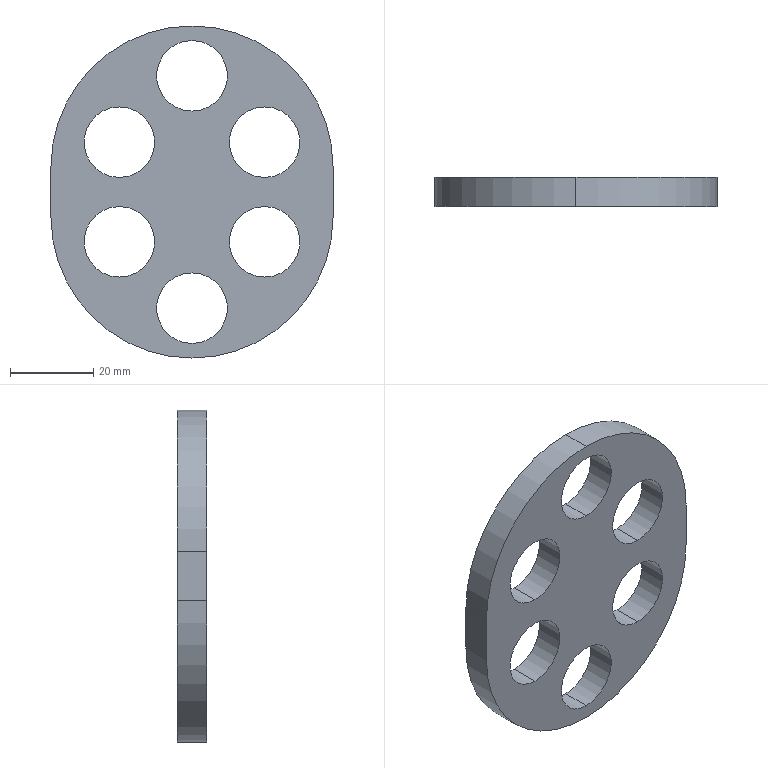Part | SolidWorks | features MirrorStock 1 | 1 solid | 19 faces | box 68 x 7 x 80 mm | volume 21601 mm3 | cylinder 15 | plane 4 | commonest cylinder face diameters 17 x12 68 x3
STEP:
#1=CARTESIAN_POINT('',(0.,7.,-36.5));
#2=VERTEX_POINT('',#1);
#3=CARTESIAN_POINT('',(0.,7.,-19.5));
#4=VERTEX_POINT('',#3);
#5=CARTESIAN_POINT('',(0.,7.,-28.));
#6=DIRECTION('',(0.,-1.,0.));
#7=DIRECTION('',(0.,0.,1.));
#8=AXIS2_PLACEMENT_3D('',#5,#6,#7);
#9=CIRCLE('',#8,8.5);
#10=EDGE_CURVE('',#2,#4,#9,.T.);
#11=ORIENTED_EDGE('',*,*,#10,.F.);
#12=CARTESIAN_POINT('',(0.,0.,-36.5));
#13=VERTEX_POINT('',#12);
#14=CARTESIAN_POINT('',(0.,7.,-36.5));
#15=DIRECTION('',(0.,-1.,0.));
#16=VECTOR('',#15,1000.);
#17=LINE('',#14,#16);
#18=EDGE_CURVE('',#2,#13,#17,.T.);
#19=ORIENTED_EDGE('',*,*,#18,.T.);
#20=CARTESIAN_POINT('',(0.,0.,-19.5));
#21=VERTEX_POINT('',#20);
#22=CARTESIAN_POINT('',(0.,0.,-28.));
#23=DIRECTION('',(0.,-1.,0.));
#24=DIRECTION('',(0.,0.,1.));
#25=AXIS2_PLACEMENT_3D('',#22,#23,#24);
#26=CIRCLE('',#25,8.5);
#27=EDGE_CURVE('',#13,#21,#26,.T.);
#28=ORIENTED_EDGE('',*,*,#27,.T.);
#29=CARTESIAN_POINT('',(0.,7.,-19.5));
#30=DIRECTION('',(0.,-1.,0.));
#31=VECTOR('',#30,1000.);
#32=LINE('',#29,#31);
#33=EDGE_CURVE('',#4,#21,#32,.T.);
#34=ORIENTED_EDGE('',*,*,#33,.F.);
#35=EDGE_LOOP('',(#11,#19,#28,#34));
#36=FACE_OUTER_BOUND('',#35,.T.);
#37=CARTESIAN_POINT('',(0.,7.,-28.));
#38=DIRECTION('',(0.,-1.,0.));
#39=DIRECTION('',(0.,0.,1.));
#40=AXIS2_PLACEMENT_3D('',#37,#38,#39);
#41=CYLINDRICAL_SURFACE('',#40,8.5);
#42=ADVANCED_FACE('',(#36),#41,.F.);
#43=CARTESIAN_POINT('',(-17.5,7.,-20.5));
#44=VERTEX_POINT('',#43);
#45=CARTESIAN_POINT('',(-17.5,7.,-3.5));
#46=VERTEX_POINT('',#45);
#47=CARTESIAN_POINT('',(-17.5,7.,-12.));
#48=DIRECTION('',(0.,-1.,0.));
#49=DIRECTION('',(0.,0.,1.));
#50=AXIS2_PLACEMENT_3D('',#47,#48,#49);
#51=CIRCLE('',#50,8.5);
#52=EDGE_CURVE('',#44,#46,#51,.T.);
#53=ORIENTED_EDGE('',*,*,#52,.F.);
#54=CARTESIAN_POINT('',(-17.5,0.,-20.5));
#55=VERTEX_POINT('',#54);
#56=CARTESIAN_POINT('',(-17.5,7.,-20.5));
#57=DIRECTION('',(0.,-1.,0.));
#58=VECTOR('',#57,1000.);
#59=LINE('',#56,#58);
#60=EDGE_CURVE('',#44,#55,#59,.T.);
#61=ORIENTED_EDGE('',*,*,#60,.T.);
#62=CARTESIAN_POINT('',(-17.5,0.,-3.5));
#63=VERTEX_POINT('',#62);
#64=CARTESIAN_POINT('',(-17.5,0.,-12.));
#65=DIRECTION('',(0.,-1.,0.));
#66=DIRECTION('',(0.,0.,1.));
#67=AXIS2_PLACEMENT_3D('',#64,#65,#66);
#68=CIRCLE('',#67,8.5);
#69=EDGE_CURVE('',#55,#63,#68,.T.);
#70=ORIENTED_EDGE('',*,*,#69,.T.);
#71=CARTESIAN_POINT('',(-17.5,7.,-3.5));
#72=DIRECTION('',(0.,-1.,0.));
#73=VECTOR('',#72,1000.);
#74=LINE('',#71,#73);
#75=EDGE_CURVE('',#46,#63,#74,.T.);
#76=ORIENTED_EDGE('',*,*,#75,.F.);
#77=EDGE_LOOP('',(#53,#61,#70,#76));
#78=FACE_OUTER_BOUND('',#77,.T.);
#79=CARTESIAN_POINT('',(-17.5,7.,-12.));
#80=DIRECTION('',(0.,-1.,0.));
#81=DIRECTION('',(0.,0.,1.));
#82=AXIS2_PLACEMENT_3D('',#79,#80,#81);
#83=CYLINDRICAL_SURFACE('',#82,8.5);
#84=ADVANCED_FACE('',(#78),#83,.F.);
#85=CARTESIAN_POINT('',(17.5,7.,-20.5));
#86=VERTEX_POINT('',#85);
#87=CARTESIAN_POINT('',(17.5,7.,-3.5));
#88=VERTEX_POINT('',#87);
#89=CARTESIAN_POINT('',(17.5,7.,-12.));
#90=DIRECTION('',(0.,-1.,0.));
#91=DIRECTION('',(0.,0.,-1.));
#92=AXIS2_PLACEMENT_3D('',#89,#90,#91);
#93=CIRCLE('',#92,8.5);
#94=EDGE_CURVE('',#86,#88,#93,.T.);
#95=ORIENTED_EDGE('',*,*,#94,.F.);
#96=CARTESIAN_POINT('',(17.5,0.,-20.5));
#97=VERTEX_POINT('',#96);
#98=CARTESIAN_POINT('',(17.5,7.,-20.5));
#99=DIRECTION('',(0.,-1.,0.));
#100=VECTOR('',#99,1000.);
#101=LINE('',#98,#100);
#102=EDGE_CURVE('',#86,#97,#101,.T.);
#103=ORIENTED_EDGE('',*,*,#102,.T.);
#104=CARTESIAN_POINT('',(17.5,0.,-3.5));
#105=VERTEX_POINT('',#104);
#106=CARTESIAN_POINT('',(17.5,0.,-12.));
#107=DIRECTION('',(0.,-1.,0.));
#108=DIRECTION('',(0.,0.,-1.));
#109=AXIS2_PLACEMENT_3D('',#106,#107,#108);
#110=CIRCLE('',#109,8.5);
#111=EDGE_CURVE('',#97,#105,#110,.T.);
#112=ORIENTED_EDGE('',*,*,#111,.T.);
#113=CARTESIAN_POINT('',(17.5,7.,-3.5));
#114=DIRECTION('',(0.,-1.,0.));
#115=VECTOR('',#114,1000.);
#116=LINE('',#113,#115);
#117=EDGE_CURVE('',#88,#105,#116,.T.);
#118=ORIENTED_EDGE('',*,*,#117,.F.);
#119=EDGE_LOOP('',(#95,#103,#112,#118));
#120=FACE_OUTER_BOUND('',#119,.T.);
#121=CARTESIAN_POINT('',(17.5,7.,-12.));
#122=DIRECTION('',(0.,-1.,0.));
#123=DIRECTION('',(0.,0.,1.));
#124=AXIS2_PLACEMENT_3D('',#121,#122,#123);
#125=CYLINDRICAL_SURFACE('',#124,8.5);
#126=ADVANCED_FACE('',(#120),#125,.F.);
#127=CARTESIAN_POINT('',(17.5,7.,3.5));
#128=VERTEX_POINT('',#127);
#129=CARTESIAN_POINT('',(17.5,7.,20.5));
#130=VERTEX_POINT('',#129);
#131=CARTESIAN_POINT('',(17.5,7.,12.));
#132=DIRECTION('',(0.,-1.,0.));
#133=DIRECTION('',(0.,0.,1.));
#134=AXIS2_PLACEMENT_3D('',#131,#132,#133);
#135=CIRCLE('',#134,8.5);
#136=EDGE_CURVE('',#128,#130,#135,.T.);
#137=ORIENTED_EDGE('',*,*,#136,.F.);
#138=CARTESIAN_POINT('',(17.5,0.,3.5));
#139=VERTEX_POINT('',#138);
#140=CARTESIAN_POINT('',(17.5,7.,3.5));
#141=DIRECTION('',(0.,-1.,0.));
#142=VECTOR('',#141,1000.);
#143=LINE('',#140,#142);
#144=EDGE_CURVE('',#128,#139,#143,.T.);
#145=ORIENTED_EDGE('',*,*,#144,.T.);
#146=CARTESIAN_POINT('',(17.5,0.,20.5));
#147=VERTEX_POINT('',#146);
#148=CARTESIAN_POINT('',(17.5,0.,12.));
#149=DIRECTION('',(0.,-1.,0.));
#150=DIRECTION('',(0.,0.,1.));
#151=AXIS2_PLACEMENT_3D('',#148,#149,#150);
#152=CIRCLE('',#151,8.5);
#153=EDGE_CURVE('',#139,#147,#152,.T.);
#154=ORIENTED_EDGE('',*,*,#153,.T.);
#155=CARTESIAN_POINT('',(17.5,7.,20.5));
#156=DIRECTION('',(0.,-1.,0.));
#157=VECTOR('',#156,1000.);
#158=LINE('',#155,#157);
#159=EDGE_CURVE('',#130,#147,#158,.T.);
#160=ORIENTED_EDGE('',*,*,#159,.F.);
#161=EDGE_LOOP('',(#137,#145,#154,#160));
#162=FACE_OUTER_BOUND('',#161,.T.);
#163=CARTESIAN_POINT('',(17.5,7.,12.));
#164=DIRECTION('',(0.,-1.,0.));
#165=DIRECTION('',(0.,0.,1.));
#166=AXIS2_PLACEMENT_3D('',#163,#164,#165);
#167=CYLINDRICAL_SURFACE('',#166,8.5);
#168=ADVANCED_FACE('',(#162),#167,.F.);
#169=CARTESIAN_POINT('',(-17.5,7.,3.5));
#170=VERTEX_POINT('',#169);
#171=CARTESIAN_POINT('',(-17.5,7.,20.5));
#172=VERTEX_POINT('',#171);
#173=CARTESIAN_POINT('',(-17.5,7.,12.));
#174=DIRECTION('',(0.,-1.,0.));
#175=DIRECTION('',(0.,0.,-1.));
#176=AXIS2_PLACEMENT_3D('',#173,#174,#175);
#177=CIRCLE('',#176,8.5);
#178=EDGE_CURVE('',#170,#172,#177,.T.);
#179=ORIENTED_EDGE('',*,*,#178,.F.);
#180=CARTESIAN_POINT('',(-17.5,0.,3.5));
#181=VERTEX_POINT('',#180);
#182=CARTESIAN_POINT('',(-17.5,7.,3.5));
#183=DIRECTION('',(0.,-1.,0.));
#184=VECTOR('',#183,1000.);
#185=LINE('',#182,#184);
#186=EDGE_CURVE('',#170,#181,#185,.T.);
#187=ORIENTED_EDGE('',*,*,#186,.T.);
#188=CARTESIAN_POINT('',(-17.5,0.,20.5));
#189=VERTEX_POINT('',#188);
#190=CARTESIAN_POINT('',(-17.5,0.,12.));
#191=DIRECTION('',(0.,-1.,0.));
#192=DIRECTION('',(0.,0.,-1.));
#193=AXIS2_PLACEMENT_3D('',#190,#191,#192);
#194=CIRCLE('',#193,8.5);
#195=EDGE_CURVE('',#181,#189,#194,.T.);
#196=ORIENTED_EDGE('',*,*,#195,.T.);
#197=CARTESIAN_POINT('',(-17.5,7.,20.5));
#198=DIRECTION('',(0.,-1.,0.));
#199=VECTOR('',#198,1000.);
#200=LINE('',#197,#199);
#201=EDGE_CURVE('',#172,#189,#200,.T.);
#202=ORIENTED_EDGE('',*,*,#201,.F.);
#203=EDGE_LOOP('',(#179,#187,#196,#202));
#204=FACE_OUTER_BOUND('',#203,.T.);
#205=CARTESIAN_POINT('',(-17.5,7.,12.));
#206=DIRECTION('',(0.,-1.,0.));
#207=DIRECTION('',(0.,0.,1.));
#208=AXIS2_PLACEMENT_3D('',#205,#206,#207);
#209=CYLINDRICAL_SURFACE('',#208,8.5);
#210=ADVANCED_FACE('',(#204),#209,.F.);
#211=CARTESIAN_POINT('',(0.,7.,19.5));
#212=VERTEX_POINT('',#211);
#213=CARTESIAN_POINT('',(0.,7.,36.5));
#214=VERTEX_POINT('',#213);
#215=CARTESIAN_POINT('',(0.,7.,28.));
#216=DIRECTION('',(0.,-1.,0.));
#217=DIRECTION('',(0.,0.,-1.));
#218=AXIS2_PLACEMENT_3D('',#215,#216,#217);
#219=CIRCLE('',#218,8.5);
#220=EDGE_CURVE('',#212,#214,#219,.T.);
#221=ORIENTED_EDGE('',*,*,#220,.F.);
#222=CARTESIAN_POINT('',(0.,0.,19.5));
#223=VERTEX_POINT('',#222);
#224=CARTESIAN_POINT('',(0.,7.,19.5));
#225=DIRECTION('',(0.,-1.,0.));
#226=VECTOR('',#225,1000.);
#227=LINE('',#224,#226);
#228=EDGE_CURVE('',#212,#223,#227,.T.);
#229=ORIENTED_EDGE('',*,*,#228,.T.);
#230=CARTESIAN_POINT('',(0.,0.,36.5));
#231=VERTEX_POINT('',#230);
#232=CARTESIAN_POINT('',(0.,0.,28.));
#233=DIRECTION('',(0.,-1.,0.));
#234=DIRECTION('',(0.,0.,-1.));
#235=AXIS2_PLACEMENT_3D('',#232,#233,#234);
#236=CIRCLE('',#235,8.5);
#237=EDGE_CURVE('',#223,#231,#236,.T.);
#238=ORIENTED_EDGE('',*,*,#237,.T.);
#239=CARTESIAN_POINT('',(0.,7.,36.5));
#240=DIRECTION('',(0.,-1.,0.));
#241=VECTOR('',#240,1000.);
#242=LINE('',#239,#241);
#243=EDGE_CURVE('',#214,#231,#242,.T.);
#244=ORIENTED_EDGE('',*,*,#243,.F.);
#245=EDGE_LOOP('',(#221,#229,#238,#244));
#246=FACE_OUTER_BOUND('',#245,.T.);
#247=CARTESIAN_POINT('',(0.,7.,28.));
#248=DIRECTION('',(0.,-1.,0.));
#249=DIRECTION('',(0.,0.,1.));
#250=AXIS2_PLACEMENT_3D('',#247,#248,#249);
#251=CYLINDRICAL_SURFACE('',#250,8.5);
#252=ADVANCED_FACE('',(#246),#251,.F.);
#253=CARTESIAN_POINT('',(34.,7.,6.));
#254=VERTEX_POINT('',#253);
#255=CARTESIAN_POINT('',(0.,7.,40.));
#256=VERTEX_POINT('',#255);
#257=CARTESIAN_POINT('',(0.,7.,6.));
#258=DIRECTION('',(0.,-1.,0.));
#259=DIRECTION('',(0.,0.,-1.));
#260=AXIS2_PLACEMENT_3D('',#257,#258,#259);
#261=CIRCLE('',#260,34.);
#262=EDGE_CURVE('',#254,#256,#261,.T.);
#263=ORIENTED_EDGE('',*,*,#262,.T.);
#264=CARTESIAN_POINT('',(0.,0.,40.));
#265=VERTEX_POINT('',#264);
#266=CARTESIAN_POINT('',(0.,7.,40.));
#267=DIRECTION('',(0.,-1.,0.));
#268=VECTOR('',#267,1000.);
#269=LINE('',#266,#268);
#270=EDGE_CURVE('',#256,#265,#269,.T.);
#271=ORIENTED_EDGE('',*,*,#270,.T.);
#272=CARTESIAN_POINT('',(34.,0.,6.));
#273=VERTEX_POINT('',#272);
#274=CARTESIAN_POINT('',(0.,0.,6.));
#275=DIRECTION('',(0.,-1.,0.));
#276=DIRECTION('',(0.,0.,-1.));
#277=AXIS2_PLACEMENT_3D('',#274,#275,#276);
#278=CIRCLE('',#277,34.);
#279=EDGE_CURVE('',#273,#265,#278,.T.);
#280=ORIENTED_EDGE('',*,*,#279,.F.);
#281=CARTESIAN_POINT('',(34.,7.,6.));
#282=DIRECTION('',(0.,-1.,0.));
#283=VECTOR('',#282,1000.);
#284=LINE('',#281,#283);
#285=EDGE_CURVE('',#254,#273,#284,.T.);
#286=ORIENTED_EDGE('',*,*,#285,.F.);
#287=EDGE_LOOP('',(#263,#271,#280,#286));
#288=FACE_OUTER_BOUND('',#287,.T.);
#289=CARTESIAN_POINT('',(0.,7.,6.));
#290=DIRECTION('',(0.,-1.,0.));
#291=DIRECTION('',(0.,0.,1.));
#292=AXIS2_PLACEMENT_3D('',#289,#290,#291);
#293=CYLINDRICAL_SURFACE('',#292,34.);
#294=ADVANCED_FACE('',(#288),#293,.T.);
#295=CARTESIAN_POINT('',(-17.5,7.,-12.));
#296=DIRECTION('',(0.,-1.,0.));
#297=DIRECTION('',(0.,0.,1.));
#298=AXIS2_PLACEMENT_3D('',#295,#296,#297);
#299=CIRCLE('',#298,8.5);
#300=EDGE_CURVE('',#46,#44,#299,.T.);
#301=ORIENTED_EDGE('',*,*,#300,.T.);
#302=ORIENTED_EDGE('',*,*,#52,.T.);
#303=EDGE_LOOP('',(#301,#302));
#304=FACE_BOUND('',#303,.T.);
#305=CARTESIAN_POINT('',(17.5,7.,12.));
#306=DIRECTION('',(0.,-1.,0.));
#307=DIRECTION('',(0.,0.,1.));
#308=AXIS2_PLACEMENT_3D('',#305,#306,#307);
#309=CIRCLE('',#308,8.5);
#310=EDGE_CURVE('',#130,#128,#309,.T.);
#311=ORIENTED_EDGE('',*,*,#310,.T.);
#312=ORIENTED_EDGE('',*,*,#136,.T.);
#313=EDGE_LOOP('',(#311,#312));
#314=FACE_BOUND('',#313,.T.);
#315=CARTESIAN_POINT('',(0.,7.,28.));
#316=DIRECTION('',(0.,-1.,0.));
#317=DIRECTION('',(0.,0.,-1.));
#318=AXIS2_PLACEMENT_3D('',#315,#316,#317);
#319=CIRCLE('',#318,8.5);
#320=EDGE_CURVE('',#214,#212,#319,.T.);
#321=ORIENTED_EDGE('',*,*,#320,.T.);
#322=ORIENTED_EDGE('',*,*,#220,.T.);
#323=EDGE_LOOP('',(#321,#322));
#324=FACE_BOUND('',#323,.T.);
#325=ORIENTED_EDGE('',*,*,#262,.F.);
#326=CARTESIAN_POINT('',(34.,7.,-6.));
#327=VERTEX_POINT('',#326);
#328=CARTESIAN_POINT('',(34.,7.,-6.));
#329=DIRECTION('',(0.,0.,1.));
#330=VECTOR('',#329,1000.);
#331=LINE('',#328,#330);
#332=EDGE_CURVE('',#327,#254,#331,.T.);
#333=ORIENTED_EDGE('',*,*,#332,.F.);
#334=CARTESIAN_POINT('',(-34.,7.,-6.));
#335=VERTEX_POINT('',#334);
#336=CARTESIAN_POINT('',(0.,7.,-6.));
#337=DIRECTION('',(0.,-1.,0.));
#338=DIRECTION('',(0.,0.,1.));
#339=AXIS2_PLACEMENT_3D('',#336,#337,#338);
#340=CIRCLE('',#339,34.);
#341=EDGE_CURVE('',#335,#327,#340,.T.);
#342=ORIENTED_EDGE('',*,*,#341,.F.);
#343=CARTESIAN_POINT('',(-34.,7.,6.));
#344=VERTEX_POINT('',#343);
#345=CARTESIAN_POINT('',(-34.,7.,-6.));
#346=DIRECTION('',(0.,0.,-1.));
#347=VECTOR('',#346,1000.);
#348=LINE('',#345,#347);
#349=EDGE_CURVE('',#344,#335,#348,.T.);
#350=ORIENTED_EDGE('',*,*,#349,.F.);
#351=CARTESIAN_POINT('',(0.,7.,6.));
#352=DIRECTION('',(0.,-1.,0.));
#353=DIRECTION('',(0.,0.,-1.));
#354=AXIS2_PLACEMENT_3D('',#351,#352,#353);
#355=CIRCLE('',#354,34.);
#356=EDGE_CURVE('',#256,#344,#355,.T.);
#357=ORIENTED_EDGE('',*,*,#356,.F.);
#358=EDGE_LOOP('',(#325,#333,#342,#350,#357));
#359=FACE_OUTER_BOUND('',#358,.T.);
#360=CARTESIAN_POINT('',(-17.5,7.,12.));
#361=DIRECTION('',(0.,-1.,0.));
#362=DIRECTION('',(0.,0.,-1.));
#363=AXIS2_PLACEMENT_3D('',#360,#361,#362);
#364=CIRCLE('',#363,8.5);
#365=EDGE_CURVE('',#172,#170,#364,.T.);
#366=ORIENTED_EDGE('',*,*,#365,.T.);
#367=ORIENTED_EDGE('',*,*,#178,.T.);
#368=EDGE_LOOP('',(#366,#367));
#369=FACE_BOUND('',#368,.T.);
#370=CARTESIAN_POINT('',(17.5,7.,-12.));
#371=DIRECTION('',(0.,-1.,0.));
#372=DIRECTION('',(0.,0.,-1.));
#373=AXIS2_PLACEMENT_3D('',#370,#371,#372);
#374=CIRCLE('',#373,8.5);
#375=EDGE_CURVE('',#88,#86,#374,.T.);
#376=ORIENTED_EDGE('',*,*,#375,.T.);
#377=ORIENTED_EDGE('',*,*,#94,.T.);
#378=EDGE_LOOP('',(#376,#377));
#379=FACE_BOUND('',#378,.T.);
#380=CARTESIAN_POINT('',(0.,7.,-28.));
#381=DIRECTION('',(0.,-1.,0.));
#382=DIRECTION('',(0.,0.,1.));
#383=AXIS2_PLACEMENT_3D('',#380,#381,#382);
#384=CIRCLE('',#383,8.5);
#385=EDGE_CURVE('',#4,#2,#384,.T.);
#386=ORIENTED_EDGE('',*,*,#385,.T.);
#387=ORIENTED_EDGE('',*,*,#10,.T.);
#388=EDGE_LOOP('',(#386,#387));
#389=FACE_BOUND('',#388,.T.);
#390=CARTESIAN_POINT('',(0.,7.,6.));
#391=DIRECTION('',(0.,1.,0.));
#392=DIRECTION('',(0.,0.,-1.));
#393=AXIS2_PLACEMENT_3D('',#390,#391,#392);
#394=PLANE('',#393);
#395=ADVANCED_FACE('',(#304,#314,#324,#359,#369,#379,#389),#394,.T.);
#396=ORIENTED_EDGE('',*,*,#279,.T.);
#397=CARTESIAN_POINT('',(-34.,0.,6.));
#398=VERTEX_POINT('',#397);
#399=CARTESIAN_POINT('',(0.,0.,6.));
#400=DIRECTION('',(0.,-1.,0.));
#401=DIRECTION('',(0.,0.,-1.));
#402=AXIS2_PLACEMENT_3D('',#399,#400,#401);
#403=CIRCLE('',#402,34.);
#404=EDGE_CURVE('',#265,#398,#403,.T.);
#405=ORIENTED_EDGE('',*,*,#404,.T.);
#406=CARTESIAN_POINT('',(-34.,0.,-6.));
#407=VERTEX_POINT('',#406);
#408=CARTESIAN_POINT('',(-34.,0.,-6.));
#409=DIRECTION('',(0.,0.,-1.));
#410=VECTOR('',#409,1000.);
#411=LINE('',#408,#410);
#412=EDGE_CURVE('',#398,#407,#411,.T.);
#413=ORIENTED_EDGE('',*,*,#412,.T.);
#414=CARTESIAN_POINT('',(34.,0.,-6.));
#415=VERTEX_POINT('',#414);
#416=CARTESIAN_POINT('',(0.,0.,-6.));
#417=DIRECTION('',(0.,-1.,0.));
#418=DIRECTION('',(0.,0.,1.));
#419=AXIS2_PLACEMENT_3D('',#416,#417,#418);
#420=CIRCLE('',#419,34.);
#421=EDGE_CURVE('',#407,#415,#420,.T.);
#422=ORIENTED_EDGE('',*,*,#421,.T.);
#423=CARTESIAN_POINT('',(34.,0.,-6.));
#424=DIRECTION('',(0.,0.,1.));
#425=VECTOR('',#424,1000.);
#426=LINE('',#423,#425);
#427=EDGE_CURVE('',#415,#273,#426,.T.);
#428=ORIENTED_EDGE('',*,*,#427,.T.);
#429=EDGE_LOOP('',(#396,#405,#413,#422,#428));
#430=FACE_OUTER_BOUND('',#429,.T.);
#431=CARTESIAN_POINT('',(0.,0.,28.));
#432=DIRECTION('',(0.,-1.,0.));
#433=DIRECTION('',(0.,0.,-1.));
#434=AXIS2_PLACEMENT_3D('',#431,#432,#433);
#435=CIRCLE('',#434,8.5);
#436=EDGE_CURVE('',#231,#223,#435,.T.);
#437=ORIENTED_EDGE('',*,*,#436,.F.);
#438=ORIENTED_EDGE('',*,*,#237,.F.);
#439=EDGE_LOOP('',(#437,#438));
#440=FACE_BOUND('',#439,.T.);
#441=CARTESIAN_POINT('',(-17.5,0.,12.));
#442=DIRECTION('',(0.,-1.,0.));
#443=DIRECTION('',(0.,0.,-1.));
#444=AXIS2_PLACEMENT_3D('',#441,#442,#443);
#445=CIRCLE('',#444,8.5);
#446=EDGE_CURVE('',#189,#181,#445,.T.);
#447=ORIENTED_EDGE('',*,*,#446,.F.);
#448=ORIENTED_EDGE('',*,*,#195,.F.);
#449=EDGE_LOOP('',(#447,#448));
#450=FACE_BOUND('',#449,.T.);
#451=CARTESIAN_POINT('',(17.5,0.,12.));
#452=DIRECTION('',(0.,-1.,0.));
#453=DIRECTION('',(0.,0.,1.));
#454=AXIS2_PLACEMENT_3D('',#451,#452,#453);
#455=CIRCLE('',#454,8.5);
#456=EDGE_CURVE('',#147,#139,#455,.T.);
#457=ORIENTED_EDGE('',*,*,#456,.F.);
#458=ORIENTED_EDGE('',*,*,#153,.F.);
#459=EDGE_LOOP('',(#457,#458));
#460=FACE_BOUND('',#459,.T.);
#461=CARTESIAN_POINT('',(17.5,0.,-12.));
#462=DIRECTION('',(0.,-1.,0.));
#463=DIRECTION('',(0.,0.,-1.));
#464=AXIS2_PLACEMENT_3D('',#461,#462,#463);
#465=CIRCLE('',#464,8.5);
#466=EDGE_CURVE('',#105,#97,#465,.T.);
#467=ORIENTED_EDGE('',*,*,#466,.F.);
#468=ORIENTED_EDGE('',*,*,#111,.F.);
#469=EDGE_LOOP('',(#467,#468));
#470=FACE_BOUND('',#469,.T.);
#471=CARTESIAN_POINT('',(-17.5,0.,-12.));
#472=DIRECTION('',(0.,-1.,0.));
#473=DIRECTION('',(0.,0.,1.));
#474=AXIS2_PLACEMENT_3D('',#471,#472,#473);
#475=CIRCLE('',#474,8.5);
#476=EDGE_CURVE('',#63,#55,#475,.T.);
#477=ORIENTED_EDGE('',*,*,#476,.F.);
#478=ORIENTED_EDGE('',*,*,#69,.F.);
#479=EDGE_LOOP('',(#477,#478));
#480=FACE_BOUND('',#479,.T.);
#481=CARTESIAN_POINT('',(0.,0.,-28.));
#482=DIRECTION('',(0.,-1.,0.));
#483=DIRECTION('',(0.,0.,1.));
#484=AXIS2_PLACEMENT_3D('',#481,#482,#483);
#485=CIRCLE('',#484,8.5);
#486=EDGE_CURVE('',#21,#13,#485,.T.);
#487=ORIENTED_EDGE('',*,*,#486,.F.);
#488=ORIENTED_EDGE('',*,*,#27,.F.);
#489=EDGE_LOOP('',(#487,#488));
#490=FACE_BOUND('',#489,.T.);
#491=CARTESIAN_POINT('',(0.,0.,6.));
#492=DIRECTION('',(0.,1.,0.));
#493=DIRECTION('',(0.,0.,-1.));
#494=AXIS2_PLACEMENT_3D('',#491,#492,#493);
#495=PLANE('',#494);
#496=ADVANCED_FACE('',(#430,#440,#450,#460,#470,#480,#490),#495,.F.);
#497=ORIENTED_EDGE('',*,*,#270,.F.);
#498=ORIENTED_EDGE('',*,*,#356,.T.);
#499=CARTESIAN_POINT('',(-34.,7.,6.));
#500=DIRECTION('',(0.,-1.,0.));
#501=VECTOR('',#500,1000.);
#502=LINE('',#499,#501);
#503=EDGE_CURVE('',#344,#398,#502,.T.);
#504=ORIENTED_EDGE('',*,*,#503,.T.);
#505=ORIENTED_EDGE('',*,*,#404,.F.);
#506=EDGE_LOOP('',(#497,#498,#504,#505));
#507=FACE_OUTER_BOUND('',#506,.T.);
#508=CARTESIAN_POINT('',(0.,7.,6.));
#509=DIRECTION('',(0.,-1.,0.));
#510=DIRECTION('',(0.,0.,1.));
#511=AXIS2_PLACEMENT_3D('',#508,#509,#510);
#512=CYLINDRICAL_SURFACE('',#511,34.);
#513=ADVANCED_FACE('',(#507),#512,.T.);
#514=ORIENTED_EDGE('',*,*,#412,.F.);
#515=ORIENTED_EDGE('',*,*,#503,.F.);
#516=ORIENTED_EDGE('',*,*,#349,.T.);
#517=CARTESIAN_POINT('',(-34.,7.,-6.));
#518=DIRECTION('',(0.,-1.,0.));
#519=VECTOR('',#518,1000.);
#520=LINE('',#517,#519);
#521=EDGE_CURVE('',#335,#407,#520,.T.);
#522=ORIENTED_EDGE('',*,*,#521,.T.);
#523=EDGE_LOOP('',(#514,#515,#516,#522));
#524=FACE_OUTER_BOUND('',#523,.T.);
#525=CARTESIAN_POINT('',(-34.,7.,-6.));
#526=DIRECTION('',(1.,0.,0.));
#527=DIRECTION('',(0.,0.,1.));
#528=AXIS2_PLACEMENT_3D('',#525,#526,#527);
#529=PLANE('',#528);
#530=ADVANCED_FACE('',(#524),#529,.F.);
#531=ORIENTED_EDGE('',*,*,#421,.F.);
#532=ORIENTED_EDGE('',*,*,#521,.F.);
#533=ORIENTED_EDGE('',*,*,#341,.T.);
#534=CARTESIAN_POINT('',(34.,7.,-6.));
#535=DIRECTION('',(0.,-1.,0.));
#536=VECTOR('',#535,1000.);
#537=LINE('',#534,#536);
#538=EDGE_CURVE('',#327,#415,#537,.T.);
#539=ORIENTED_EDGE('',*,*,#538,.T.);
#540=EDGE_LOOP('',(#531,#532,#533,#539));
#541=FACE_OUTER_BOUND('',#540,.T.);
#542=CARTESIAN_POINT('',(0.,7.,-6.));
#543=DIRECTION('',(0.,-1.,0.));
#544=DIRECTION('',(0.,0.,1.));
#545=AXIS2_PLACEMENT_3D('',#542,#543,#544);
#546=CYLINDRICAL_SURFACE('',#545,34.);
#547=ADVANCED_FACE('',(#541),#546,.T.);
#548=ORIENTED_EDGE('',*,*,#427,.F.);
#549=ORIENTED_EDGE('',*,*,#538,.F.);
#550=ORIENTED_EDGE('',*,*,#332,.T.);
#551=ORIENTED_EDGE('',*,*,#285,.T.);
#552=EDGE_LOOP('',(#548,#549,#550,#551));
#553=FACE_OUTER_BOUND('',#552,.T.);
#554=CARTESIAN_POINT('',(34.,7.,-6.));
#555=DIRECTION('',(-1.,0.,0.));
#556=DIRECTION('',(0.,0.,-1.));
#557=AXIS2_PLACEMENT_3D('',#554,#555,#556);
#558=PLANE('',#557);
#559=ADVANCED_FACE('',(#553),#558,.F.);
#560=ORIENTED_EDGE('',*,*,#228,.F.);
#561=ORIENTED_EDGE('',*,*,#320,.F.);
#562=ORIENTED_EDGE('',*,*,#243,.T.);
#563=ORIENTED_EDGE('',*,*,#436,.T.);
#564=EDGE_LOOP('',(#560,#561,#562,#563));
#565=FACE_OUTER_BOUND('',#564,.T.);
#566=CARTESIAN_POINT('',(0.,7.,28.));
#567=DIRECTION('',(0.,-1.,0.));
#568=DIRECTION('',(0.,0.,1.));
#569=AXIS2_PLACEMENT_3D('',#566,#567,#568);
#570=CYLINDRICAL_SURFACE('',#569,8.5);
#571=ADVANCED_FACE('',(#565),#570,.F.);
#572=ORIENTED_EDGE('',*,*,#186,.F.);
#573=ORIENTED_EDGE('',*,*,#365,.F.);
#574=ORIENTED_EDGE('',*,*,#201,.T.);
#575=ORIENTED_EDGE('',*,*,#446,.T.);
#576=EDGE_LOOP('',(#572,#573,#574,#575));
#577=FACE_OUTER_BOUND('',#576,.T.);
#578=CARTESIAN_POINT('',(-17.5,7.,12.));
#579=DIRECTION('',(0.,-1.,0.));
#580=DIRECTION('',(0.,0.,1.));
#581=AXIS2_PLACEMENT_3D('',#578,#579,#580);
#582=CYLINDRICAL_SURFACE('',#581,8.5);
#583=ADVANCED_FACE('',(#577),#582,.F.);
#584=ORIENTED_EDGE('',*,*,#144,.F.);
#585=ORIENTED_EDGE('',*,*,#310,.F.);
#586=ORIENTED_EDGE('',*,*,#159,.T.);
#587=ORIENTED_EDGE('',*,*,#456,.T.);
#588=EDGE_LOOP('',(#584,#585,#586,#587));
#589=FACE_OUTER_BOUND('',#588,.T.);
#590=CARTESIAN_POINT('',(17.5,7.,12.));
#591=DIRECTION('',(0.,-1.,0.));
#592=DIRECTION('',(0.,0.,1.));
#593=AXIS2_PLACEMENT_3D('',#590,#591,#592);
#594=CYLINDRICAL_SURFACE('',#593,8.5);
#595=ADVANCED_FACE('',(#589),#594,.F.);
#596=ORIENTED_EDGE('',*,*,#102,.F.);
#597=ORIENTED_EDGE('',*,*,#375,.F.);
#598=ORIENTED_EDGE('',*,*,#117,.T.);
#599=ORIENTED_EDGE('',*,*,#466,.T.);
#600=EDGE_LOOP('',(#596,#597,#598,#599));
#601=FACE_OUTER_BOUND('',#600,.T.);
#602=CARTESIAN_POINT('',(17.5,7.,-12.));
#603=DIRECTION('',(0.,-1.,0.));
#604=DIRECTION('',(0.,0.,1.));
#605=AXIS2_PLACEMENT_3D('',#602,#603,#604);
#606=CYLINDRICAL_SURFACE('',#605,8.5);
#607=ADVANCED_FACE('',(#601),#606,.F.);
#608=ORIENTED_EDGE('',*,*,#60,.F.);
#609=ORIENTED_EDGE('',*,*,#300,.F.);
#610=ORIENTED_EDGE('',*,*,#75,.T.);
#611=ORIENTED_EDGE('',*,*,#476,.T.);
#612=EDGE_LOOP('',(#608,#609,#610,#611));
#613=FACE_OUTER_BOUND('',#612,.T.);
#614=CARTESIAN_POINT('',(-17.5,7.,-12.));
#615=DIRECTION('',(0.,-1.,0.));
#616=DIRECTION('',(0.,0.,1.));
#617=AXIS2_PLACEMENT_3D('',#614,#615,#616);
#618=CYLINDRICAL_SURFACE('',#617,8.5);
#619=ADVANCED_FACE('',(#613),#618,.F.);
#620=ORIENTED_EDGE('',*,*,#18,.F.);
#621=ORIENTED_EDGE('',*,*,#385,.F.);
#622=ORIENTED_EDGE('',*,*,#33,.T.);
#623=ORIENTED_EDGE('',*,*,#486,.T.);
#624=EDGE_LOOP('',(#620,#621,#622,#623));
#625=FACE_OUTER_BOUND('',#624,.T.);
#626=CARTESIAN_POINT('',(0.,7.,-28.));
#627=DIRECTION('',(0.,-1.,0.));
#628=DIRECTION('',(0.,0.,1.));
#629=AXIS2_PLACEMENT_3D('',#626,#627,#628);
#630=CYLINDRICAL_SURFACE('',#629,8.5);
#631=ADVANCED_FACE('',(#625),#630,.F.);
#632=CLOSED_SHELL('',(#42,#84,#126,#168,#210,#252,#294,#395,#496,#513,#530,#547,#559,#571,#583,#595,#607,#619,#631));
#633=MANIFOLD_SOLID_BREP('',#632);
#634=CARTESIAN_POINT('',(0.,0.,0.));
#635=DIRECTION('',(0.,0.,1.));
#636=DIRECTION('',(1.,0.,0.));
#637=AXIS2_PLACEMENT_3D('',#634,#635,#636);
#638=(LENGTH_UNIT()NAMED_UNIT(*)SI_UNIT(.MILLI.,.METRE.));
#639=UNCERTAINTY_MEASURE_WITH_UNIT(LENGTH_MEASURE(0.00001),#638,'','');
#640=(NAMED_UNIT(*)PLANE_ANGLE_UNIT()SI_UNIT($,.RADIAN.));
#641=(NAMED_UNIT(*)SI_UNIT($,.STERADIAN.)SOLID_ANGLE_UNIT());
#642=(GEOMETRIC_REPRESENTATION_CONTEXT(3)GLOBAL_UNCERTAINTY_ASSIGNED_CONTEXT((#639))GLOBAL_UNIT_ASSIGNED_CONTEXT((#638,#640,#641))REPRESENTATION_CONTEXT('',''));
#643=ADVANCED_BREP_SHAPE_REPRESENTATION('',(#633,#637),#642);